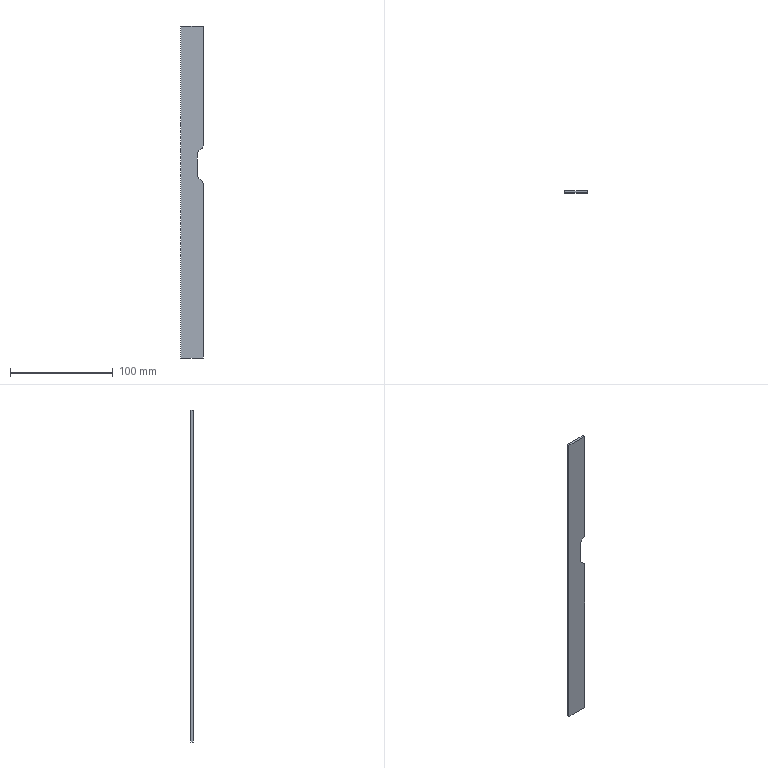Part | SolidWorks | features Fillet 1, FlatPattern 1, SMBaseFlange 1, SheetMetal 1 | 1 solid | 14 faces | box 22 x 2.3 x 323 mm | volume 15944 mm3 | plane 10 | cylinder 4 | commonest cylinder face diameters 10 x4
STEP:
#1=CARTESIAN_POINT('',(0.,0.,0.));
#2=VERTEX_POINT('',#1);
#3=CARTESIAN_POINT('',(0.,0.,323.));
#4=VERTEX_POINT('',#3);
#5=CARTESIAN_POINT('',(0.,0.,0.));
#6=DIRECTION('',(0.,0.,1.));
#7=VECTOR('',#6,1000.);
#8=LINE('',#5,#7);
#9=EDGE_CURVE('',#2,#4,#8,.T.);
#10=ORIENTED_EDGE('',*,*,#9,.F.);
#11=CARTESIAN_POINT('',(0.,-2.3,0.));
#12=VERTEX_POINT('',#11);
#13=CARTESIAN_POINT('',(0.,-2.3,0.));
#14=DIRECTION('',(0.,1.,0.));
#15=VECTOR('',#14,1000.);
#16=LINE('',#13,#15);
#17=EDGE_CURVE('',#12,#2,#16,.T.);
#18=ORIENTED_EDGE('',*,*,#17,.F.);
#19=CARTESIAN_POINT('',(0.,-2.3,323.));
#20=VERTEX_POINT('',#19);
#21=CARTESIAN_POINT('',(0.,-2.3,0.));
#22=DIRECTION('',(0.,0.,1.));
#23=VECTOR('',#22,1000.);
#24=LINE('',#21,#23);
#25=EDGE_CURVE('',#12,#20,#24,.T.);
#26=ORIENTED_EDGE('',*,*,#25,.T.);
#27=CARTESIAN_POINT('',(0.,-2.3,323.));
#28=DIRECTION('',(0.,1.,0.));
#29=VECTOR('',#28,1000.);
#30=LINE('',#27,#29);
#31=EDGE_CURVE('',#20,#4,#30,.T.);
#32=ORIENTED_EDGE('',*,*,#31,.T.);
#33=EDGE_LOOP('',(#10,#18,#26,#32));
#34=FACE_OUTER_BOUND('',#33,.T.);
#35=CARTESIAN_POINT('',(0.,-2.3,0.));
#36=DIRECTION('',(-1.,0.,0.));
#37=DIRECTION('',(0.,0.,1.));
#38=AXIS2_PLACEMENT_3D('',#35,#36,#37);
#39=PLANE('',#38);
#40=ADVANCED_FACE('',(#34),#39,.T.);
#41=CARTESIAN_POINT('',(22.,0.,0.));
#42=VERTEX_POINT('',#41);
#43=CARTESIAN_POINT('',(0.,0.,0.));
#44=DIRECTION('',(-1.,0.,0.));
#45=VECTOR('',#44,1000.);
#46=LINE('',#43,#45);
#47=EDGE_CURVE('',#42,#2,#46,.T.);
#48=ORIENTED_EDGE('',*,*,#47,.F.);
#49=CARTESIAN_POINT('',(22.,-2.3,0.));
#50=VERTEX_POINT('',#49);
#51=CARTESIAN_POINT('',(22.,-2.3,0.));
#52=DIRECTION('',(0.,1.,0.));
#53=VECTOR('',#52,1000.);
#54=LINE('',#51,#53);
#55=EDGE_CURVE('',#50,#42,#54,.T.);
#56=ORIENTED_EDGE('',*,*,#55,.F.);
#57=CARTESIAN_POINT('',(0.,-2.3,0.));
#58=DIRECTION('',(-1.,0.,0.));
#59=VECTOR('',#58,1000.);
#60=LINE('',#57,#59);
#61=EDGE_CURVE('',#50,#12,#60,.T.);
#62=ORIENTED_EDGE('',*,*,#61,.T.);
#63=ORIENTED_EDGE('',*,*,#17,.T.);
#64=EDGE_LOOP('',(#48,#56,#62,#63));
#65=FACE_OUTER_BOUND('',#64,.T.);
#66=CARTESIAN_POINT('',(0.,-2.3,0.));
#67=DIRECTION('',(0.,0.,-1.));
#68=DIRECTION('',(-1.,0.,0.));
#69=AXIS2_PLACEMENT_3D('',#66,#67,#68);
#70=PLANE('',#69);
#71=ADVANCED_FACE('',(#65),#70,.T.);
#72=CARTESIAN_POINT('',(22.,0.,168.658));
#73=VERTEX_POINT('',#72);
#74=CARTESIAN_POINT('',(22.,0.,0.));
#75=DIRECTION('',(0.,0.,-1.));
#76=VECTOR('',#75,1000.);
#77=LINE('',#74,#76);
#78=EDGE_CURVE('',#73,#42,#77,.T.);
#79=ORIENTED_EDGE('',*,*,#78,.F.);
#80=CARTESIAN_POINT('',(22.,-2.3,168.658));
#81=VERTEX_POINT('',#80);
#82=CARTESIAN_POINT('',(22.,-2.3,168.658));
#83=DIRECTION('',(0.,-1.,0.));
#84=VECTOR('',#83,1000.);
#85=LINE('',#82,#84);
#86=EDGE_CURVE('',#73,#81,#85,.T.);
#87=ORIENTED_EDGE('',*,*,#86,.T.);
#88=CARTESIAN_POINT('',(22.,-2.3,0.));
#89=DIRECTION('',(0.,0.,-1.));
#90=VECTOR('',#89,1000.);
#91=LINE('',#88,#90);
#92=EDGE_CURVE('',#81,#50,#91,.T.);
#93=ORIENTED_EDGE('',*,*,#92,.T.);
#94=ORIENTED_EDGE('',*,*,#55,.T.);
#95=EDGE_LOOP('',(#79,#87,#93,#94));
#96=FACE_OUTER_BOUND('',#95,.T.);
#97=CARTESIAN_POINT('',(22.,-2.3,0.));
#98=DIRECTION('',(1.,0.,0.));
#99=DIRECTION('',(0.,0.,-1.));
#100=AXIS2_PLACEMENT_3D('',#97,#98,#99);
#101=PLANE('',#100);
#102=ADVANCED_FACE('',(#96),#101,.T.);
#103=CARTESIAN_POINT('',(17.799,0.,174.501));
#104=VERTEX_POINT('',#103);
#105=CARTESIAN_POINT('',(20.201,0.,172.499));
#106=VERTEX_POINT('',#105);
#107=CARTESIAN_POINT('',(16.,0.,176.));
#108=DIRECTION('',(0.7682,0.,-0.6402));
#109=VECTOR('',#108,1000.);
#110=LINE('',#107,#109);
#111=EDGE_CURVE('',#104,#106,#110,.T.);
#112=ORIENTED_EDGE('',*,*,#111,.F.);
#113=CARTESIAN_POINT('',(17.799,-2.3,174.501));
#114=VERTEX_POINT('',#113);
#115=CARTESIAN_POINT('',(17.799,-2.3,174.501));
#116=DIRECTION('',(0.,-1.,0.));
#117=VECTOR('',#116,1000.);
#118=LINE('',#115,#117);
#119=EDGE_CURVE('',#104,#114,#118,.T.);
#120=ORIENTED_EDGE('',*,*,#119,.T.);
#121=CARTESIAN_POINT('',(20.201,-2.3,172.499));
#122=VERTEX_POINT('',#121);
#123=CARTESIAN_POINT('',(16.,-2.3,176.));
#124=DIRECTION('',(0.7682,0.,-0.6402));
#125=VECTOR('',#124,1000.);
#126=LINE('',#123,#125);
#127=EDGE_CURVE('',#114,#122,#126,.T.);
#128=ORIENTED_EDGE('',*,*,#127,.T.);
#129=CARTESIAN_POINT('',(20.201,-2.3,172.499));
#130=DIRECTION('',(0.,1.,0.));
#131=VECTOR('',#130,1000.);
#132=LINE('',#129,#131);
#133=EDGE_CURVE('',#122,#106,#132,.T.);
#134=ORIENTED_EDGE('',*,*,#133,.T.);
#135=EDGE_LOOP('',(#112,#120,#128,#134));
#136=FACE_OUTER_BOUND('',#135,.T.);
#137=CARTESIAN_POINT('',(16.,-2.3,176.));
#138=DIRECTION('',(0.6402,0.,0.7682));
#139=DIRECTION('',(0.7682,0.,-0.6402));
#140=AXIS2_PLACEMENT_3D('',#137,#138,#139);
#141=PLANE('',#140);
#142=ADVANCED_FACE('',(#136),#141,.T.);
#143=CARTESIAN_POINT('',(16.,0.,197.658));
#144=VERTEX_POINT('',#143);
#145=CARTESIAN_POINT('',(16.,0.,178.342));
#146=VERTEX_POINT('',#145);
#147=CARTESIAN_POINT('',(16.,0.,176.));
#148=DIRECTION('',(0.,0.,-1.));
#149=VECTOR('',#148,1000.);
#150=LINE('',#147,#149);
#151=EDGE_CURVE('',#144,#146,#150,.T.);
#152=ORIENTED_EDGE('',*,*,#151,.F.);
#153=CARTESIAN_POINT('',(16.,-2.3,197.658));
#154=VERTEX_POINT('',#153);
#155=CARTESIAN_POINT('',(16.,-2.3,197.658));
#156=DIRECTION('',(0.,-1.,0.));
#157=VECTOR('',#156,1000.);
#158=LINE('',#155,#157);
#159=EDGE_CURVE('',#144,#154,#158,.T.);
#160=ORIENTED_EDGE('',*,*,#159,.T.);
#161=CARTESIAN_POINT('',(16.,-2.3,178.342));
#162=VERTEX_POINT('',#161);
#163=CARTESIAN_POINT('',(16.,-2.3,176.));
#164=DIRECTION('',(0.,0.,-1.));
#165=VECTOR('',#164,1000.);
#166=LINE('',#163,#165);
#167=EDGE_CURVE('',#154,#162,#166,.T.);
#168=ORIENTED_EDGE('',*,*,#167,.T.);
#169=CARTESIAN_POINT('',(16.,0.,178.342));
#170=DIRECTION('',(0.,1.,0.));
#171=VECTOR('',#170,1000.);
#172=LINE('',#169,#171);
#173=EDGE_CURVE('',#162,#146,#172,.T.);
#174=ORIENTED_EDGE('',*,*,#173,.T.);
#175=EDGE_LOOP('',(#152,#160,#168,#174));
#176=FACE_OUTER_BOUND('',#175,.T.);
#177=CARTESIAN_POINT('',(16.,-2.3,176.));
#178=DIRECTION('',(1.,0.,0.));
#179=DIRECTION('',(0.,0.,-1.));
#180=AXIS2_PLACEMENT_3D('',#177,#178,#179);
#181=PLANE('',#180);
#182=ADVANCED_FACE('',(#176),#181,.T.);
#183=CARTESIAN_POINT('',(20.201,0.,203.501));
#184=VERTEX_POINT('',#183);
#185=CARTESIAN_POINT('',(17.799,0.,201.499));
#186=VERTEX_POINT('',#185);
#187=CARTESIAN_POINT('',(16.,0.,200.));
#188=DIRECTION('',(-0.7682,0.,-0.6402));
#189=VECTOR('',#188,1000.);
#190=LINE('',#187,#189);
#191=EDGE_CURVE('',#184,#186,#190,.T.);
#192=ORIENTED_EDGE('',*,*,#191,.F.);
#193=CARTESIAN_POINT('',(20.201,-2.3,203.501));
#194=VERTEX_POINT('',#193);
#195=CARTESIAN_POINT('',(20.201,-2.3,203.501));
#196=DIRECTION('',(0.,-1.,0.));
#197=VECTOR('',#196,1000.);
#198=LINE('',#195,#197);
#199=EDGE_CURVE('',#184,#194,#198,.T.);
#200=ORIENTED_EDGE('',*,*,#199,.T.);
#201=CARTESIAN_POINT('',(17.799,-2.3,201.499));
#202=VERTEX_POINT('',#201);
#203=CARTESIAN_POINT('',(16.,-2.3,200.));
#204=DIRECTION('',(-0.7682,0.,-0.6402));
#205=VECTOR('',#204,1000.);
#206=LINE('',#203,#205);
#207=EDGE_CURVE('',#194,#202,#206,.T.);
#208=ORIENTED_EDGE('',*,*,#207,.T.);
#209=CARTESIAN_POINT('',(17.799,0.,201.499));
#210=DIRECTION('',(0.,1.,0.));
#211=VECTOR('',#210,1000.);
#212=LINE('',#209,#211);
#213=EDGE_CURVE('',#202,#186,#212,.T.);
#214=ORIENTED_EDGE('',*,*,#213,.T.);
#215=EDGE_LOOP('',(#192,#200,#208,#214));
#216=FACE_OUTER_BOUND('',#215,.T.);
#217=CARTESIAN_POINT('',(16.,-2.3,200.));
#218=DIRECTION('',(0.6402,0.,-0.7682));
#219=DIRECTION('',(-0.7682,0.,-0.6402));
#220=AXIS2_PLACEMENT_3D('',#217,#218,#219);
#221=PLANE('',#220);
#222=ADVANCED_FACE('',(#216),#221,.T.);
#223=CARTESIAN_POINT('',(22.,-2.3,323.));
#224=VERTEX_POINT('',#223);
#225=CARTESIAN_POINT('',(22.,-2.3,207.342));
#226=VERTEX_POINT('',#225);
#227=CARTESIAN_POINT('',(22.,-2.3,205.));
#228=DIRECTION('',(0.,0.,-1.));
#229=VECTOR('',#228,1000.);
#230=LINE('',#227,#229);
#231=EDGE_CURVE('',#224,#226,#230,.T.);
#232=ORIENTED_EDGE('',*,*,#231,.T.);
#233=CARTESIAN_POINT('',(22.,0.,207.342));
#234=VERTEX_POINT('',#233);
#235=CARTESIAN_POINT('',(22.,-2.3,207.342));
#236=DIRECTION('',(0.,1.,0.));
#237=VECTOR('',#236,1000.);
#238=LINE('',#235,#237);
#239=EDGE_CURVE('',#226,#234,#238,.T.);
#240=ORIENTED_EDGE('',*,*,#239,.T.);
#241=CARTESIAN_POINT('',(22.,0.,323.));
#242=VERTEX_POINT('',#241);
#243=CARTESIAN_POINT('',(22.,0.,205.));
#244=DIRECTION('',(0.,0.,-1.));
#245=VECTOR('',#244,1000.);
#246=LINE('',#243,#245);
#247=EDGE_CURVE('',#242,#234,#246,.T.);
#248=ORIENTED_EDGE('',*,*,#247,.F.);
#249=CARTESIAN_POINT('',(22.,-2.3,323.));
#250=DIRECTION('',(0.,1.,0.));
#251=VECTOR('',#250,1000.);
#252=LINE('',#249,#251);
#253=EDGE_CURVE('',#224,#242,#252,.T.);
#254=ORIENTED_EDGE('',*,*,#253,.F.);
#255=EDGE_LOOP('',(#232,#240,#248,#254));
#256=FACE_OUTER_BOUND('',#255,.T.);
#257=CARTESIAN_POINT('',(22.,-2.3,205.));
#258=DIRECTION('',(1.,0.,0.));
#259=DIRECTION('',(0.,0.,-1.));
#260=AXIS2_PLACEMENT_3D('',#257,#258,#259);
#261=PLANE('',#260);
#262=ADVANCED_FACE('',(#256),#261,.T.);
#263=CARTESIAN_POINT('',(0.,0.,323.));
#264=DIRECTION('',(1.,0.,0.));
#265=VECTOR('',#264,1000.);
#266=LINE('',#263,#265);
#267=EDGE_CURVE('',#4,#242,#266,.T.);
#268=ORIENTED_EDGE('',*,*,#267,.F.);
#269=ORIENTED_EDGE('',*,*,#31,.F.);
#270=CARTESIAN_POINT('',(0.,-2.3,323.));
#271=DIRECTION('',(1.,0.,0.));
#272=VECTOR('',#271,1000.);
#273=LINE('',#270,#272);
#274=EDGE_CURVE('',#20,#224,#273,.T.);
#275=ORIENTED_EDGE('',*,*,#274,.T.);
#276=ORIENTED_EDGE('',*,*,#253,.T.);
#277=EDGE_LOOP('',(#268,#269,#275,#276));
#278=FACE_OUTER_BOUND('',#277,.T.);
#279=CARTESIAN_POINT('',(0.,-2.3,323.));
#280=DIRECTION('',(0.,0.,1.));
#281=DIRECTION('',(1.,0.,0.));
#282=AXIS2_PLACEMENT_3D('',#279,#280,#281);
#283=PLANE('',#282);
#284=ADVANCED_FACE('',(#278),#283,.T.);
#285=ORIENTED_EDGE('',*,*,#207,.F.);
#286=CARTESIAN_POINT('',(17.,-2.3,207.342));
#287=DIRECTION('',(0.,-1.,0.));
#288=DIRECTION('',(0.,0.,1.));
#289=AXIS2_PLACEMENT_3D('',#286,#287,#288);
#290=CIRCLE('',#289,5.);
#291=EDGE_CURVE('',#194,#226,#290,.T.);
#292=ORIENTED_EDGE('',*,*,#291,.T.);
#293=ORIENTED_EDGE('',*,*,#231,.F.);
#294=ORIENTED_EDGE('',*,*,#274,.F.);
#295=ORIENTED_EDGE('',*,*,#25,.F.);
#296=ORIENTED_EDGE('',*,*,#61,.F.);
#297=ORIENTED_EDGE('',*,*,#92,.F.);
#298=CARTESIAN_POINT('',(17.,-2.3,168.658));
#299=DIRECTION('',(0.,-1.,0.));
#300=DIRECTION('',(0.,0.,1.));
#301=AXIS2_PLACEMENT_3D('',#298,#299,#300);
#302=CIRCLE('',#301,5.);
#303=EDGE_CURVE('',#81,#122,#302,.T.);
#304=ORIENTED_EDGE('',*,*,#303,.T.);
#305=ORIENTED_EDGE('',*,*,#127,.F.);
#306=CARTESIAN_POINT('',(21.,-2.3,178.342));
#307=DIRECTION('',(0.,1.,0.));
#308=DIRECTION('',(0.,0.,1.));
#309=AXIS2_PLACEMENT_3D('',#306,#307,#308);
#310=CIRCLE('',#309,5.);
#311=EDGE_CURVE('',#114,#162,#310,.T.);
#312=ORIENTED_EDGE('',*,*,#311,.T.);
#313=ORIENTED_EDGE('',*,*,#167,.F.);
#314=CARTESIAN_POINT('',(21.,-2.3,197.658));
#315=DIRECTION('',(0.,1.,0.));
#316=DIRECTION('',(0.,0.,1.));
#317=AXIS2_PLACEMENT_3D('',#314,#315,#316);
#318=CIRCLE('',#317,5.);
#319=EDGE_CURVE('',#154,#202,#318,.T.);
#320=ORIENTED_EDGE('',*,*,#319,.T.);
#321=EDGE_LOOP('',(#285,#292,#293,#294,#295,#296,#297,#304,#305,#312,#313,#320));
#322=FACE_OUTER_BOUND('',#321,.T.);
#323=CARTESIAN_POINT('',(0.,-2.3,0.));
#324=DIRECTION('',(0.,1.,0.));
#325=DIRECTION('',(0.,0.,1.));
#326=AXIS2_PLACEMENT_3D('',#323,#324,#325);
#327=PLANE('',#326);
#328=ADVANCED_FACE('',(#322),#327,.F.);
#329=ORIENTED_EDGE('',*,*,#247,.T.);
#330=CARTESIAN_POINT('',(17.,0.,207.342));
#331=DIRECTION('',(0.,1.,0.));
#332=DIRECTION('',(0.,0.,1.));
#333=AXIS2_PLACEMENT_3D('',#330,#331,#332);
#334=CIRCLE('',#333,5.);
#335=EDGE_CURVE('',#234,#184,#334,.T.);
#336=ORIENTED_EDGE('',*,*,#335,.T.);
#337=ORIENTED_EDGE('',*,*,#191,.T.);
#338=CARTESIAN_POINT('',(21.,0.,197.658));
#339=DIRECTION('',(0.,-1.,0.));
#340=DIRECTION('',(0.,0.,1.));
#341=AXIS2_PLACEMENT_3D('',#338,#339,#340);
#342=CIRCLE('',#341,5.);
#343=EDGE_CURVE('',#186,#144,#342,.T.);
#344=ORIENTED_EDGE('',*,*,#343,.T.);
#345=ORIENTED_EDGE('',*,*,#151,.T.);
#346=CARTESIAN_POINT('',(21.,0.,178.342));
#347=DIRECTION('',(0.,-1.,0.));
#348=DIRECTION('',(0.,0.,1.));
#349=AXIS2_PLACEMENT_3D('',#346,#347,#348);
#350=CIRCLE('',#349,5.);
#351=EDGE_CURVE('',#146,#104,#350,.T.);
#352=ORIENTED_EDGE('',*,*,#351,.T.);
#353=ORIENTED_EDGE('',*,*,#111,.T.);
#354=CARTESIAN_POINT('',(17.,0.,168.658));
#355=DIRECTION('',(0.,1.,0.));
#356=DIRECTION('',(0.,0.,1.));
#357=AXIS2_PLACEMENT_3D('',#354,#355,#356);
#358=CIRCLE('',#357,5.);
#359=EDGE_CURVE('',#106,#73,#358,.T.);
#360=ORIENTED_EDGE('',*,*,#359,.T.);
#361=ORIENTED_EDGE('',*,*,#78,.T.);
#362=ORIENTED_EDGE('',*,*,#47,.T.);
#363=ORIENTED_EDGE('',*,*,#9,.T.);
#364=ORIENTED_EDGE('',*,*,#267,.T.);
#365=EDGE_LOOP('',(#329,#336,#337,#344,#345,#352,#353,#360,#361,#362,#363,#364));
#366=FACE_OUTER_BOUND('',#365,.T.);
#367=CARTESIAN_POINT('',(0.,0.,0.));
#368=DIRECTION('',(0.,1.,0.));
#369=DIRECTION('',(0.,0.,1.));
#370=AXIS2_PLACEMENT_3D('',#367,#368,#369);
#371=PLANE('',#370);
#372=ADVANCED_FACE('',(#366),#371,.T.);
#373=ORIENTED_EDGE('',*,*,#291,.F.);
#374=ORIENTED_EDGE('',*,*,#199,.F.);
#375=ORIENTED_EDGE('',*,*,#335,.F.);
#376=ORIENTED_EDGE('',*,*,#239,.F.);
#377=EDGE_LOOP('',(#373,#374,#375,#376));
#378=FACE_OUTER_BOUND('',#377,.T.);
#379=CARTESIAN_POINT('',(17.,-2.3,207.342));
#380=DIRECTION('',(0.,1.,0.));
#381=DIRECTION('',(0.,0.,1.));
#382=AXIS2_PLACEMENT_3D('',#379,#380,#381);
#383=CYLINDRICAL_SURFACE('',#382,5.);
#384=ADVANCED_FACE('',(#378),#383,.T.);
#385=ORIENTED_EDGE('',*,*,#319,.F.);
#386=ORIENTED_EDGE('',*,*,#159,.F.);
#387=ORIENTED_EDGE('',*,*,#343,.F.);
#388=ORIENTED_EDGE('',*,*,#213,.F.);
#389=EDGE_LOOP('',(#385,#386,#387,#388));
#390=FACE_OUTER_BOUND('',#389,.T.);
#391=CARTESIAN_POINT('',(21.,-2.3,197.658));
#392=DIRECTION('',(0.,-1.,0.));
#393=DIRECTION('',(0.,0.,-1.));
#394=AXIS2_PLACEMENT_3D('',#391,#392,#393);
#395=CYLINDRICAL_SURFACE('',#394,5.);
#396=ADVANCED_FACE('',(#390),#395,.F.);
#397=ORIENTED_EDGE('',*,*,#311,.F.);
#398=ORIENTED_EDGE('',*,*,#119,.F.);
#399=ORIENTED_EDGE('',*,*,#351,.F.);
#400=ORIENTED_EDGE('',*,*,#173,.F.);
#401=EDGE_LOOP('',(#397,#398,#399,#400));
#402=FACE_OUTER_BOUND('',#401,.T.);
#403=CARTESIAN_POINT('',(21.,-2.3,178.342));
#404=DIRECTION('',(0.,-1.,0.));
#405=DIRECTION('',(0.,0.,-1.));
#406=AXIS2_PLACEMENT_3D('',#403,#404,#405);
#407=CYLINDRICAL_SURFACE('',#406,5.);
#408=ADVANCED_FACE('',(#402),#407,.F.);
#409=ORIENTED_EDGE('',*,*,#303,.F.);
#410=ORIENTED_EDGE('',*,*,#86,.F.);
#411=ORIENTED_EDGE('',*,*,#359,.F.);
#412=ORIENTED_EDGE('',*,*,#133,.F.);
#413=EDGE_LOOP('',(#409,#410,#411,#412));
#414=FACE_OUTER_BOUND('',#413,.T.);
#415=CARTESIAN_POINT('',(17.,-2.3,168.658));
#416=DIRECTION('',(0.,1.,0.));
#417=DIRECTION('',(0.,0.,1.));
#418=AXIS2_PLACEMENT_3D('',#415,#416,#417);
#419=CYLINDRICAL_SURFACE('',#418,5.);
#420=ADVANCED_FACE('',(#414),#419,.T.);
#421=CLOSED_SHELL('',(#40,#71,#102,#142,#182,#222,#262,#284,#328,#372,#384,#396,#408,#420));
#422=MANIFOLD_SOLID_BREP('',#421);
#423=CARTESIAN_POINT('',(0.,0.,0.));
#424=DIRECTION('',(0.,0.,1.));
#425=DIRECTION('',(1.,0.,0.));
#426=AXIS2_PLACEMENT_3D('',#423,#424,#425);
#427=(LENGTH_UNIT()NAMED_UNIT(*)SI_UNIT(.MILLI.,.METRE.));
#428=UNCERTAINTY_MEASURE_WITH_UNIT(LENGTH_MEASURE(0.00001),#427,'','');
#429=(NAMED_UNIT(*)PLANE_ANGLE_UNIT()SI_UNIT($,.RADIAN.));
#430=(NAMED_UNIT(*)SI_UNIT($,.STERADIAN.)SOLID_ANGLE_UNIT());
#431=(GEOMETRIC_REPRESENTATION_CONTEXT(3)GLOBAL_UNCERTAINTY_ASSIGNED_CONTEXT((#428))GLOBAL_UNIT_ASSIGNED_CONTEXT((#427,#429,#430))REPRESENTATION_CONTEXT('',''));
#432=ADVANCED_BREP_SHAPE_REPRESENTATION('',(#422,#426),#431);